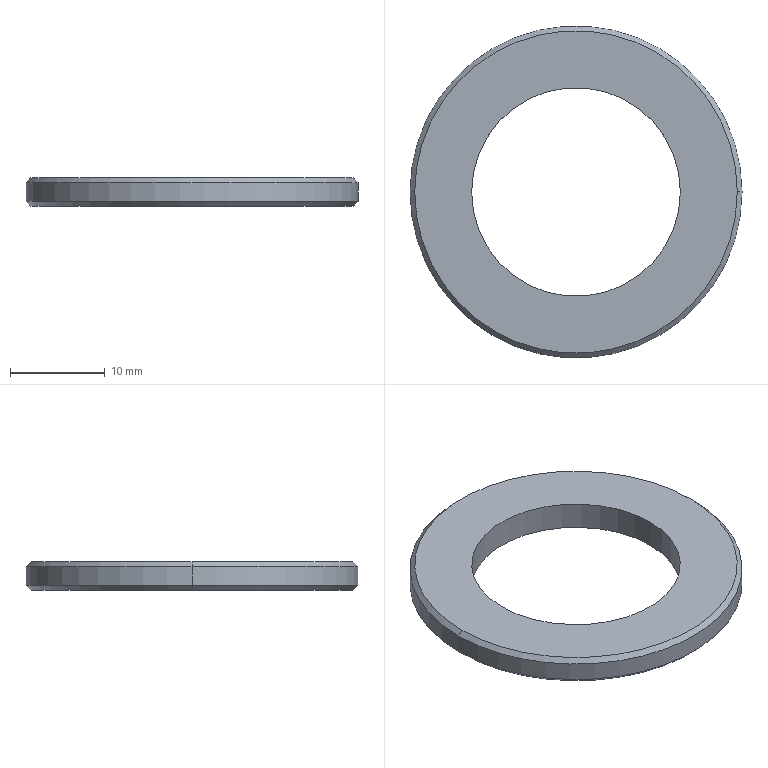Part | SolidWorks | features Chamfer 1, Extrusion 1 | 1 solid | 10 faces | box 35 x 35 x 3 mm | volume 1719 mm3 | cone 4 | cylinder 4 | plane 2 | commonest cylinder face diameters 22 x2 35 x2
STEP:
#1=CARTESIAN_POINT('',(17.,0.,3.));
#2=VERTEX_POINT('',#1);
#3=CARTESIAN_POINT('',(-17.,0.,3.));
#4=VERTEX_POINT('',#3);
#5=CARTESIAN_POINT('',(0.,0.,3.));
#6=DIRECTION('',(0.,0.,1.));
#7=DIRECTION('',(1.,0.,0.));
#8=AXIS2_PLACEMENT_3D('',#5,#6,#7);
#9=CIRCLE('',#8,17.);
#10=EDGE_CURVE('',#2,#4,#9,.T.);
#11=ORIENTED_EDGE('',*,*,#10,.F.);
#12=CARTESIAN_POINT('',(17.5,0.,2.5));
#13=VERTEX_POINT('',#12);
#14=CARTESIAN_POINT('',(17.,0.,3.));
#15=DIRECTION('',(0.7071,0.,-0.7071));
#16=VECTOR('',#15,1000.);
#17=LINE('',#14,#16);
#18=EDGE_CURVE('',#2,#13,#17,.T.);
#19=ORIENTED_EDGE('',*,*,#18,.T.);
#20=CARTESIAN_POINT('',(-17.5,0.,2.5));
#21=VERTEX_POINT('',#20);
#22=CARTESIAN_POINT('',(0.,0.,2.5));
#23=DIRECTION('',(0.,0.,-1.));
#24=DIRECTION('',(1.,0.,0.));
#25=AXIS2_PLACEMENT_3D('',#22,#23,#24);
#26=CIRCLE('',#25,17.5);
#27=EDGE_CURVE('',#21,#13,#26,.T.);
#28=ORIENTED_EDGE('',*,*,#27,.F.);
#29=CARTESIAN_POINT('',(-17.,0.,3.));
#30=DIRECTION('',(-0.7071,0.,-0.7071));
#31=VECTOR('',#30,1000.);
#32=LINE('',#29,#31);
#33=EDGE_CURVE('',#4,#21,#32,.T.);
#34=ORIENTED_EDGE('',*,*,#33,.F.);
#35=EDGE_LOOP('',(#11,#19,#28,#34));
#36=FACE_OUTER_BOUND('',#35,.T.);
#37=CARTESIAN_POINT('',(0.,0.,3.));
#38=DIRECTION('',(0.,0.,-1.));
#39=DIRECTION('',(-1.,0.,0.));
#40=AXIS2_PLACEMENT_3D('',#37,#38,#39);
#41=CONICAL_SURFACE('',#40,17.,0.7854);
#42=ADVANCED_FACE('',(#36),#41,.T.);
#43=CARTESIAN_POINT('',(-17.,0.,0.));
#44=VERTEX_POINT('',#43);
#45=CARTESIAN_POINT('',(17.,0.,0.));
#46=VERTEX_POINT('',#45);
#47=CARTESIAN_POINT('',(0.,0.,0.));
#48=DIRECTION('',(0.,0.,-1.));
#49=DIRECTION('',(1.,0.,0.));
#50=AXIS2_PLACEMENT_3D('',#47,#48,#49);
#51=CIRCLE('',#50,17.);
#52=EDGE_CURVE('',#44,#46,#51,.T.);
#53=ORIENTED_EDGE('',*,*,#52,.F.);
#54=CARTESIAN_POINT('',(-17.5,0.,0.5));
#55=VERTEX_POINT('',#54);
#56=CARTESIAN_POINT('',(-17.5,0.,0.5));
#57=DIRECTION('',(-0.7071,0.,0.7071));
#58=VECTOR('',#57,1000.);
#59=LINE('',#56,#58);
#60=EDGE_CURVE('',#44,#55,#59,.T.);
#61=ORIENTED_EDGE('',*,*,#60,.T.);
#62=CARTESIAN_POINT('',(17.5,0.,0.5));
#63=VERTEX_POINT('',#62);
#64=CARTESIAN_POINT('',(0.,0.,0.5));
#65=DIRECTION('',(0.,0.,1.));
#66=DIRECTION('',(1.,0.,0.));
#67=AXIS2_PLACEMENT_3D('',#64,#65,#66);
#68=CIRCLE('',#67,17.5);
#69=EDGE_CURVE('',#63,#55,#68,.T.);
#70=ORIENTED_EDGE('',*,*,#69,.F.);
#71=CARTESIAN_POINT('',(17.5,0.,0.5));
#72=DIRECTION('',(0.7071,0.,0.7071));
#73=VECTOR('',#72,1000.);
#74=LINE('',#71,#73);
#75=EDGE_CURVE('',#46,#63,#74,.T.);
#76=ORIENTED_EDGE('',*,*,#75,.F.);
#77=EDGE_LOOP('',(#53,#61,#70,#76));
#78=FACE_OUTER_BOUND('',#77,.T.);
#79=CARTESIAN_POINT('',(0.,0.,0.5));
#80=DIRECTION('',(0.,0.,1.));
#81=DIRECTION('',(1.,0.,0.));
#82=AXIS2_PLACEMENT_3D('',#79,#80,#81);
#83=CONICAL_SURFACE('',#82,17.5,0.7854);
#84=ADVANCED_FACE('',(#78),#83,.T.);
#85=CARTESIAN_POINT('',(-11.,0.,3.));
#86=VERTEX_POINT('',#85);
#87=CARTESIAN_POINT('',(11.,0.,3.));
#88=VERTEX_POINT('',#87);
#89=CARTESIAN_POINT('',(0.,0.,3.));
#90=DIRECTION('',(0.,0.,1.));
#91=DIRECTION('',(1.,0.,0.));
#92=AXIS2_PLACEMENT_3D('',#89,#90,#91);
#93=CIRCLE('',#92,11.);
#94=EDGE_CURVE('',#86,#88,#93,.T.);
#95=ORIENTED_EDGE('',*,*,#94,.T.);
#96=CARTESIAN_POINT('',(11.,0.,0.));
#97=VERTEX_POINT('',#96);
#98=CARTESIAN_POINT('',(11.,0.,3.));
#99=DIRECTION('',(0.,0.,-1.));
#100=VECTOR('',#99,1000.);
#101=LINE('',#98,#100);
#102=EDGE_CURVE('',#88,#97,#101,.T.);
#103=ORIENTED_EDGE('',*,*,#102,.T.);
#104=CARTESIAN_POINT('',(-11.,0.,0.));
#105=VERTEX_POINT('',#104);
#106=CARTESIAN_POINT('',(0.,0.,0.));
#107=DIRECTION('',(0.,0.,1.));
#108=DIRECTION('',(1.,0.,0.));
#109=AXIS2_PLACEMENT_3D('',#106,#107,#108);
#110=CIRCLE('',#109,11.);
#111=EDGE_CURVE('',#105,#97,#110,.T.);
#112=ORIENTED_EDGE('',*,*,#111,.F.);
#113=CARTESIAN_POINT('',(-11.,0.,3.));
#114=DIRECTION('',(0.,0.,-1.));
#115=VECTOR('',#114,1000.);
#116=LINE('',#113,#115);
#117=EDGE_CURVE('',#86,#105,#116,.T.);
#118=ORIENTED_EDGE('',*,*,#117,.F.);
#119=EDGE_LOOP('',(#95,#103,#112,#118));
#120=FACE_OUTER_BOUND('',#119,.T.);
#121=CARTESIAN_POINT('',(0.,0.,3.));
#122=DIRECTION('',(0.,0.,-1.));
#123=DIRECTION('',(-1.,0.,0.));
#124=AXIS2_PLACEMENT_3D('',#121,#122,#123);
#125=CYLINDRICAL_SURFACE('',#124,11.);
#126=ADVANCED_FACE('',(#120),#125,.F.);
#127=ORIENTED_EDGE('',*,*,#27,.T.);
#128=CARTESIAN_POINT('',(17.5,0.,3.));
#129=DIRECTION('',(0.,0.,-1.));
#130=VECTOR('',#129,1000.);
#131=LINE('',#128,#130);
#132=EDGE_CURVE('',#13,#63,#131,.T.);
#133=ORIENTED_EDGE('',*,*,#132,.T.);
#134=ORIENTED_EDGE('',*,*,#69,.T.);
#135=CARTESIAN_POINT('',(-17.5,0.,3.));
#136=DIRECTION('',(0.,0.,-1.));
#137=VECTOR('',#136,1000.);
#138=LINE('',#135,#137);
#139=EDGE_CURVE('',#21,#55,#138,.T.);
#140=ORIENTED_EDGE('',*,*,#139,.F.);
#141=EDGE_LOOP('',(#127,#133,#134,#140));
#142=FACE_OUTER_BOUND('',#141,.T.);
#143=CARTESIAN_POINT('',(0.,0.,3.));
#144=DIRECTION('',(0.,0.,-1.));
#145=DIRECTION('',(-1.,0.,0.));
#146=AXIS2_PLACEMENT_3D('',#143,#144,#145);
#147=CYLINDRICAL_SURFACE('',#146,17.5);
#148=ADVANCED_FACE('',(#142),#147,.T.);
#149=CARTESIAN_POINT('',(0.,0.,3.));
#150=DIRECTION('',(0.,0.,1.));
#151=DIRECTION('',(1.,0.,0.));
#152=AXIS2_PLACEMENT_3D('',#149,#150,#151);
#153=CIRCLE('',#152,17.);
#154=EDGE_CURVE('',#4,#2,#153,.T.);
#155=ORIENTED_EDGE('',*,*,#154,.T.);
#156=ORIENTED_EDGE('',*,*,#10,.T.);
#157=EDGE_LOOP('',(#155,#156));
#158=FACE_OUTER_BOUND('',#157,.T.);
#159=ORIENTED_EDGE('',*,*,#94,.F.);
#160=CARTESIAN_POINT('',(0.,0.,3.));
#161=DIRECTION('',(0.,0.,1.));
#162=DIRECTION('',(1.,0.,0.));
#163=AXIS2_PLACEMENT_3D('',#160,#161,#162);
#164=CIRCLE('',#163,11.);
#165=EDGE_CURVE('',#88,#86,#164,.T.);
#166=ORIENTED_EDGE('',*,*,#165,.F.);
#167=EDGE_LOOP('',(#159,#166));
#168=FACE_BOUND('',#167,.T.);
#169=CARTESIAN_POINT('',(0.,0.,3.));
#170=DIRECTION('',(0.,0.,1.));
#171=DIRECTION('',(1.,0.,0.));
#172=AXIS2_PLACEMENT_3D('',#169,#170,#171);
#173=PLANE('',#172);
#174=ADVANCED_FACE('',(#158,#168),#173,.T.);
#175=CARTESIAN_POINT('',(0.,0.,0.));
#176=DIRECTION('',(0.,0.,-1.));
#177=DIRECTION('',(1.,0.,0.));
#178=AXIS2_PLACEMENT_3D('',#175,#176,#177);
#179=CIRCLE('',#178,17.);
#180=EDGE_CURVE('',#46,#44,#179,.T.);
#181=ORIENTED_EDGE('',*,*,#180,.T.);
#182=ORIENTED_EDGE('',*,*,#52,.T.);
#183=EDGE_LOOP('',(#181,#182));
#184=FACE_OUTER_BOUND('',#183,.T.);
#185=ORIENTED_EDGE('',*,*,#111,.T.);
#186=CARTESIAN_POINT('',(0.,0.,0.));
#187=DIRECTION('',(0.,0.,1.));
#188=DIRECTION('',(1.,0.,0.));
#189=AXIS2_PLACEMENT_3D('',#186,#187,#188);
#190=CIRCLE('',#189,11.);
#191=EDGE_CURVE('',#97,#105,#190,.T.);
#192=ORIENTED_EDGE('',*,*,#191,.T.);
#193=EDGE_LOOP('',(#185,#192));
#194=FACE_BOUND('',#193,.T.);
#195=CARTESIAN_POINT('',(0.,0.,0.));
#196=DIRECTION('',(0.,0.,1.));
#197=DIRECTION('',(1.,0.,0.));
#198=AXIS2_PLACEMENT_3D('',#195,#196,#197);
#199=PLANE('',#198);
#200=ADVANCED_FACE('',(#184,#194),#199,.F.);
#201=ORIENTED_EDGE('',*,*,#132,.F.);
#202=CARTESIAN_POINT('',(0.,0.,2.5));
#203=DIRECTION('',(0.,0.,-1.));
#204=DIRECTION('',(1.,0.,0.));
#205=AXIS2_PLACEMENT_3D('',#202,#203,#204);
#206=CIRCLE('',#205,17.5);
#207=EDGE_CURVE('',#13,#21,#206,.T.);
#208=ORIENTED_EDGE('',*,*,#207,.T.);
#209=ORIENTED_EDGE('',*,*,#139,.T.);
#210=CARTESIAN_POINT('',(0.,0.,0.5));
#211=DIRECTION('',(0.,0.,1.));
#212=DIRECTION('',(1.,0.,0.));
#213=AXIS2_PLACEMENT_3D('',#210,#211,#212);
#214=CIRCLE('',#213,17.5);
#215=EDGE_CURVE('',#55,#63,#214,.T.);
#216=ORIENTED_EDGE('',*,*,#215,.T.);
#217=EDGE_LOOP('',(#201,#208,#209,#216));
#218=FACE_OUTER_BOUND('',#217,.T.);
#219=CARTESIAN_POINT('',(0.,0.,3.));
#220=DIRECTION('',(0.,0.,-1.));
#221=DIRECTION('',(-1.,0.,0.));
#222=AXIS2_PLACEMENT_3D('',#219,#220,#221);
#223=CYLINDRICAL_SURFACE('',#222,17.5);
#224=ADVANCED_FACE('',(#218),#223,.T.);
#225=ORIENTED_EDGE('',*,*,#102,.F.);
#226=ORIENTED_EDGE('',*,*,#165,.T.);
#227=ORIENTED_EDGE('',*,*,#117,.T.);
#228=ORIENTED_EDGE('',*,*,#191,.F.);
#229=EDGE_LOOP('',(#225,#226,#227,#228));
#230=FACE_OUTER_BOUND('',#229,.T.);
#231=CARTESIAN_POINT('',(0.,0.,3.));
#232=DIRECTION('',(0.,0.,-1.));
#233=DIRECTION('',(-1.,0.,0.));
#234=AXIS2_PLACEMENT_3D('',#231,#232,#233);
#235=CYLINDRICAL_SURFACE('',#234,11.);
#236=ADVANCED_FACE('',(#230),#235,.F.);
#237=ORIENTED_EDGE('',*,*,#60,.F.);
#238=ORIENTED_EDGE('',*,*,#180,.F.);
#239=ORIENTED_EDGE('',*,*,#75,.T.);
#240=ORIENTED_EDGE('',*,*,#215,.F.);
#241=EDGE_LOOP('',(#237,#238,#239,#240));
#242=FACE_OUTER_BOUND('',#241,.T.);
#243=CARTESIAN_POINT('',(0.,0.,0.5));
#244=DIRECTION('',(0.,0.,1.));
#245=DIRECTION('',(1.,0.,0.));
#246=AXIS2_PLACEMENT_3D('',#243,#244,#245);
#247=CONICAL_SURFACE('',#246,17.5,0.7854);
#248=ADVANCED_FACE('',(#242),#247,.T.);
#249=ORIENTED_EDGE('',*,*,#18,.F.);
#250=ORIENTED_EDGE('',*,*,#154,.F.);
#251=ORIENTED_EDGE('',*,*,#33,.T.);
#252=ORIENTED_EDGE('',*,*,#207,.F.);
#253=EDGE_LOOP('',(#249,#250,#251,#252));
#254=FACE_OUTER_BOUND('',#253,.T.);
#255=CARTESIAN_POINT('',(0.,0.,3.));
#256=DIRECTION('',(0.,0.,-1.));
#257=DIRECTION('',(-1.,0.,0.));
#258=AXIS2_PLACEMENT_3D('',#255,#256,#257);
#259=CONICAL_SURFACE('',#258,17.,0.7854);
#260=ADVANCED_FACE('',(#254),#259,.T.);
#261=CLOSED_SHELL('',(#42,#84,#126,#148,#174,#200,#224,#236,#248,#260));
#262=MANIFOLD_SOLID_BREP('',#261);
#263=CARTESIAN_POINT('',(0.,0.,0.));
#264=DIRECTION('',(0.,0.,1.));
#265=DIRECTION('',(1.,0.,0.));
#266=AXIS2_PLACEMENT_3D('',#263,#264,#265);
#267=(LENGTH_UNIT()NAMED_UNIT(*)SI_UNIT(.MILLI.,.METRE.));
#268=UNCERTAINTY_MEASURE_WITH_UNIT(LENGTH_MEASURE(0.00001),#267,'','');
#269=(NAMED_UNIT(*)PLANE_ANGLE_UNIT()SI_UNIT($,.RADIAN.));
#270=(NAMED_UNIT(*)SI_UNIT($,.STERADIAN.)SOLID_ANGLE_UNIT());
#271=(GEOMETRIC_REPRESENTATION_CONTEXT(3)GLOBAL_UNCERTAINTY_ASSIGNED_CONTEXT((#268))GLOBAL_UNIT_ASSIGNED_CONTEXT((#267,#269,#270))REPRESENTATION_CONTEXT('',''));
#272=ADVANCED_BREP_SHAPE_REPRESENTATION('',(#262,#266),#271);